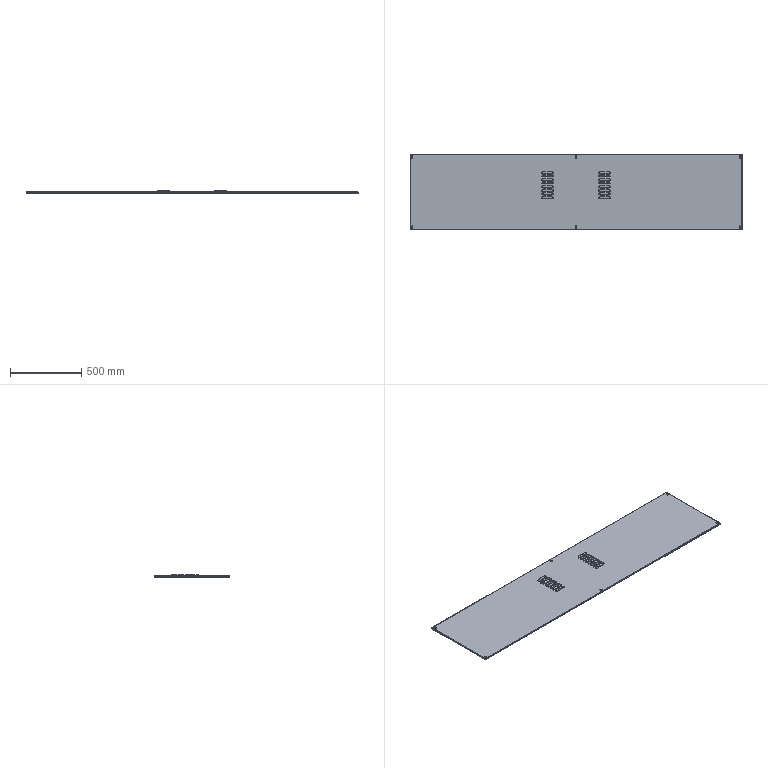Part | NX | features BREP 1 | 1 solid | 251 faces | box 2334 x 534 x 18 mm | volume 2079847 mm3 | cylinder 112 | plane 103 | torus 32 | sphere 4 | commonest cylinder face diameters 6 x54 28 x32 12 x18 2 x8